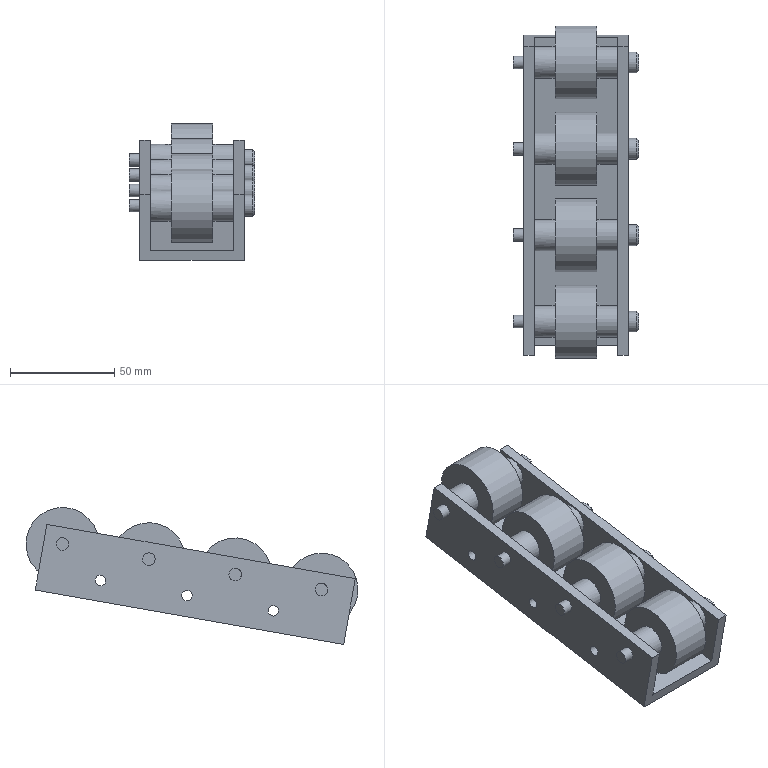Part | NX | features solid 2 | 1 solid | 56 faces | box 60 x 159.086 x 65.62 mm | volume 170595 mm3 | plane 26 | cylinder 26 | cone 4 | commonest cylinder face diameters 15 x8 5 x6 6 x4 10 x4 35 x4
STEP:
#1=CARTESIAN_POINT('',(-385.,-375.046,1.735));
#2=VERTEX_POINT('',#1);
#3=CARTESIAN_POINT('',(-385.,-374.612,-0.7271));
#4=DIRECTION('',(-1.,0.,0.));
#5=DIRECTION('',(0.,-0.1736,0.9848));
#6=AXIS2_PLACEMENT_3D('',#3,#4,#5);
#7=CIRCLE('',#6,2.5);
#8=EDGE_CURVE('',#2,#2,#7,.F.);
#9=ORIENTED_EDGE('',*,*,#8,.F.);
#10=EDGE_LOOP('',(#9));
#11=FACE_BOUND('',#10,.T.);
#12=CARTESIAN_POINT('',(-385.,-357.664,24.093));
#13=VERTEX_POINT('',#12);
#14=CARTESIAN_POINT('',(-385.,-356.362,16.707));
#15=DIRECTION('',(-1.,0.,0.));
#16=DIRECTION('',(0.,-0.1736,0.9848));
#17=AXIS2_PLACEMENT_3D('',#14,#15,#16);
#18=CIRCLE('',#17,7.5);
#19=EDGE_CURVE('',#13,#13,#18,.F.);
#20=ORIENTED_EDGE('',*,*,#19,.F.);
#21=EDGE_LOOP('',(#20));
#22=FACE_BOUND('',#21,.T.);
#23=CARTESIAN_POINT('',(-385.,-440.388,9.506));
#24=VERTEX_POINT('',#23);
#25=CARTESIAN_POINT('',(-385.,-439.086,2.12));
#26=DIRECTION('',(-1.,0.,0.));
#27=DIRECTION('',(0.,-0.1736,0.9848));
#28=AXIS2_PLACEMENT_3D('',#25,#26,#27);
#29=CIRCLE('',#28,7.5);
#30=EDGE_CURVE('',#24,#24,#29,.F.);
#31=ORIENTED_EDGE('',*,*,#30,.F.);
#32=EDGE_LOOP('',(#31));
#33=FACE_BOUND('',#32,.T.);
#34=CARTESIAN_POINT('',(-385.,-302.837,6.851));
#35=VERTEX_POINT('',#34);
#36=CARTESIAN_POINT('',(-385.,-307.526,33.441));
#37=VERTEX_POINT('',#36);
#38=CARTESIAN_POINT('',(-385.,-301.969,1.927));
#39=DIRECTION('',(0.,-0.1736,0.9848));
#40=VECTOR('',#39,1000.);
#41=LINE('',#38,#40);
#42=EDGE_CURVE('',#35,#37,#41,.T.);
#43=ORIENTED_EDGE('',*,*,#42,.T.);
#44=CARTESIAN_POINT('',(-385.,-455.247,7.394));
#45=VERTEX_POINT('',#44);
#46=CARTESIAN_POINT('',(-385.,-455.247,7.394));
#47=DIRECTION('',(0.,0.9848,0.1736));
#48=VECTOR('',#47,1000.);
#49=LINE('',#46,#48);
#50=EDGE_CURVE('',#45,#37,#49,.T.);
#51=ORIENTED_EDGE('',*,*,#50,.F.);
#52=CARTESIAN_POINT('',(-385.,-450.559,-19.196));
#53=VERTEX_POINT('',#52);
#54=CARTESIAN_POINT('',(-385.,-449.69,-24.12));
#55=DIRECTION('',(0.,-0.1736,0.9848));
#56=VECTOR('',#55,1000.);
#57=LINE('',#54,#56);
#58=EDGE_CURVE('',#53,#45,#57,.T.);
#59=ORIENTED_EDGE('',*,*,#58,.F.);
#60=CARTESIAN_POINT('',(-385.,-450.559,-19.196));
#61=DIRECTION('',(0.,0.9848,0.1736));
#62=VECTOR('',#61,1000.);
#63=LINE('',#60,#62);
#64=EDGE_CURVE('',#53,#35,#63,.T.);
#65=ORIENTED_EDGE('',*,*,#64,.T.);
#66=EDGE_LOOP('',(#43,#51,#59,#65));
#67=FACE_BOUND('',#66,.T.);
#68=CARTESIAN_POINT('',(-385.,-416.408,-5.558));
#69=VERTEX_POINT('',#68);
#70=CARTESIAN_POINT('',(-385.,-415.974,-8.02));
#71=DIRECTION('',(-1.,0.,0.));
#72=DIRECTION('',(0.,-0.1736,0.9848));
#73=AXIS2_PLACEMENT_3D('',#70,#71,#72);
#74=CIRCLE('',#73,2.5);
#75=EDGE_CURVE('',#69,#69,#74,.F.);
#76=ORIENTED_EDGE('',*,*,#75,.F.);
#77=EDGE_LOOP('',(#76));
#78=FACE_BOUND('',#77,.T.);
#79=CARTESIAN_POINT('',(-385.,-399.026,16.8));
#80=VERTEX_POINT('',#79);
#81=CARTESIAN_POINT('',(-385.,-397.724,9.414));
#82=DIRECTION('',(-1.,0.,0.));
#83=DIRECTION('',(0.,-0.1736,0.9848));
#84=AXIS2_PLACEMENT_3D('',#81,#82,#83);
#85=CIRCLE('',#84,7.5);
#86=EDGE_CURVE('',#80,#80,#85,.F.);
#87=ORIENTED_EDGE('',*,*,#86,.F.);
#88=EDGE_LOOP('',(#87));
#89=FACE_BOUND('',#88,.T.);
#90=CARTESIAN_POINT('',(-385.,-316.302,31.386));
#91=VERTEX_POINT('',#90);
#92=CARTESIAN_POINT('',(-385.,-315.,24.));
#93=DIRECTION('',(-1.,0.,0.));
#94=DIRECTION('',(0.,-0.1736,0.9848));
#95=AXIS2_PLACEMENT_3D('',#92,#93,#94);
#96=CIRCLE('',#95,7.5);
#97=EDGE_CURVE('',#91,#91,#96,.F.);
#98=ORIENTED_EDGE('',*,*,#97,.F.);
#99=EDGE_LOOP('',(#98));
#100=FACE_BOUND('',#99,.T.);
#101=CARTESIAN_POINT('',(-385.,-333.684,9.028));
#102=VERTEX_POINT('',#101);
#103=CARTESIAN_POINT('',(-385.,-333.25,6.566));
#104=DIRECTION('',(-1.,0.,0.));
#105=DIRECTION('',(0.,-0.1736,0.9848));
#106=AXIS2_PLACEMENT_3D('',#103,#104,#105);
#107=CIRCLE('',#106,2.5);
#108=EDGE_CURVE('',#102,#102,#107,.F.);
#109=ORIENTED_EDGE('',*,*,#108,.F.);
#110=EDGE_LOOP('',(#109));
#111=FACE_BOUND('',#110,.T.);
#112=CARTESIAN_POINT('',(-385.,-449.69,-24.12));
#113=DIRECTION('',(-1.,0.,0.));
#114=DIRECTION('',(0.,-0.1736,0.9848));
#115=AXIS2_PLACEMENT_3D('',#112,#113,#114);
#116=PLANE('',#115);
#117=ADVANCED_FACE('',(#11,#22,#33,#67,#78,#89,#100,#111),#116,.F.);
#118=CARTESIAN_POINT('',(-345.,-374.178,-3.189));
#119=VERTEX_POINT('',#118);
#120=CARTESIAN_POINT('',(-345.,-374.612,-0.7271));
#121=DIRECTION('',(1.,0.,0.));
#122=DIRECTION('',(0.,0.1736,-0.9848));
#123=AXIS2_PLACEMENT_3D('',#120,#121,#122);
#124=CIRCLE('',#123,2.5);
#125=EDGE_CURVE('',#119,#119,#124,.F.);
#126=ORIENTED_EDGE('',*,*,#125,.F.);
#127=EDGE_LOOP('',(#126));
#128=FACE_BOUND('',#127,.T.);
#129=CARTESIAN_POINT('',(-345.,-307.614,25.302));
#130=VERTEX_POINT('',#129);
#131=CARTESIAN_POINT('',(-345.,-315.,24.));
#132=DIRECTION('',(-1.,0.,0.));
#133=DIRECTION('',(0.,0.9848,0.1736));
#134=AXIS2_PLACEMENT_3D('',#131,#132,#133);
#135=CIRCLE('',#134,7.5);
#136=EDGE_CURVE('',#130,#130,#135,.T.);
#137=ORIENTED_EDGE('',*,*,#136,.F.);
#138=EDGE_LOOP('',(#137));
#139=FACE_BOUND('',#138,.T.);
#140=CARTESIAN_POINT('',(-345.,-348.976,18.009));
#141=VERTEX_POINT('',#140);
#142=CARTESIAN_POINT('',(-345.,-356.362,16.707));
#143=DIRECTION('',(-1.,0.,0.));
#144=DIRECTION('',(0.,0.9848,0.1736));
#145=AXIS2_PLACEMENT_3D('',#142,#143,#144);
#146=CIRCLE('',#145,7.5);
#147=EDGE_CURVE('',#141,#141,#146,.T.);
#148=ORIENTED_EDGE('',*,*,#147,.F.);
#149=EDGE_LOOP('',(#148));
#150=FACE_BOUND('',#149,.T.);
#151=CARTESIAN_POINT('',(-345.,-390.338,10.716));
#152=VERTEX_POINT('',#151);
#153=CARTESIAN_POINT('',(-345.,-397.724,9.414));
#154=DIRECTION('',(-1.,0.,0.));
#155=DIRECTION('',(0.,0.9848,0.1736));
#156=AXIS2_PLACEMENT_3D('',#153,#154,#155);
#157=CIRCLE('',#156,7.5);
#158=EDGE_CURVE('',#152,#152,#157,.T.);
#159=ORIENTED_EDGE('',*,*,#158,.F.);
#160=EDGE_LOOP('',(#159));
#161=FACE_BOUND('',#160,.T.);
#162=CARTESIAN_POINT('',(-345.,-415.54,-10.482));
#163=VERTEX_POINT('',#162);
#164=CARTESIAN_POINT('',(-345.,-415.974,-8.02));
#165=DIRECTION('',(1.,0.,0.));
#166=DIRECTION('',(0.,0.1736,-0.9848));
#167=AXIS2_PLACEMENT_3D('',#164,#165,#166);
#168=CIRCLE('',#167,2.5);
#169=EDGE_CURVE('',#163,#163,#168,.F.);
#170=ORIENTED_EDGE('',*,*,#169,.F.);
#171=EDGE_LOOP('',(#170));
#172=FACE_BOUND('',#171,.T.);
#173=CARTESIAN_POINT('',(-345.,-431.7,3.423));
#174=VERTEX_POINT('',#173);
#175=CARTESIAN_POINT('',(-345.,-439.086,2.12));
#176=DIRECTION('',(-1.,0.,0.));
#177=DIRECTION('',(0.,0.9848,0.1736));
#178=AXIS2_PLACEMENT_3D('',#175,#176,#177);
#179=CIRCLE('',#178,7.5);
#180=EDGE_CURVE('',#174,#174,#179,.T.);
#181=ORIENTED_EDGE('',*,*,#180,.F.);
#182=EDGE_LOOP('',(#181));
#183=FACE_BOUND('',#182,.T.);
#184=CARTESIAN_POINT('',(-345.,-307.526,33.441));
#185=VERTEX_POINT('',#184);
#186=CARTESIAN_POINT('',(-345.,-302.837,6.851));
#187=VERTEX_POINT('',#186);
#188=CARTESIAN_POINT('',(-345.,-307.526,33.441));
#189=DIRECTION('',(0.,0.1736,-0.9848));
#190=VECTOR('',#189,1000.);
#191=LINE('',#188,#190);
#192=EDGE_CURVE('',#185,#187,#191,.T.);
#193=ORIENTED_EDGE('',*,*,#192,.T.);
#194=CARTESIAN_POINT('',(-345.,-450.559,-19.196));
#195=VERTEX_POINT('',#194);
#196=CARTESIAN_POINT('',(-345.,-450.559,-19.196));
#197=DIRECTION('',(0.,0.9848,0.1736));
#198=VECTOR('',#197,1000.);
#199=LINE('',#196,#198);
#200=EDGE_CURVE('',#195,#187,#199,.T.);
#201=ORIENTED_EDGE('',*,*,#200,.F.);
#202=CARTESIAN_POINT('',(-345.,-455.247,7.394));
#203=VERTEX_POINT('',#202);
#204=CARTESIAN_POINT('',(-345.,-455.247,7.394));
#205=DIRECTION('',(0.,0.1736,-0.9848));
#206=VECTOR('',#205,1000.);
#207=LINE('',#204,#206);
#208=EDGE_CURVE('',#203,#195,#207,.T.);
#209=ORIENTED_EDGE('',*,*,#208,.F.);
#210=CARTESIAN_POINT('',(-345.,-455.247,7.394));
#211=DIRECTION('',(0.,0.9848,0.1736));
#212=VECTOR('',#211,1000.);
#213=LINE('',#210,#212);
#214=EDGE_CURVE('',#203,#185,#213,.T.);
#215=ORIENTED_EDGE('',*,*,#214,.T.);
#216=EDGE_LOOP('',(#193,#201,#209,#215));
#217=FACE_BOUND('',#216,.T.);
#218=CARTESIAN_POINT('',(-345.,-332.816,4.104));
#219=VERTEX_POINT('',#218);
#220=CARTESIAN_POINT('',(-345.,-333.25,6.566));
#221=DIRECTION('',(1.,0.,0.));
#222=DIRECTION('',(0.,0.1736,-0.9848));
#223=AXIS2_PLACEMENT_3D('',#220,#221,#222);
#224=CIRCLE('',#223,2.5);
#225=EDGE_CURVE('',#219,#219,#224,.F.);
#226=ORIENTED_EDGE('',*,*,#225,.F.);
#227=EDGE_LOOP('',(#226));
#228=FACE_BOUND('',#227,.T.);
#229=CARTESIAN_POINT('',(-345.,-455.247,7.394));
#230=DIRECTION('',(1.,0.,0.));
#231=DIRECTION('',(0.,0.1736,-0.9848));
#232=AXIS2_PLACEMENT_3D('',#229,#230,#231);
#233=PLANE('',#232);
#234=ADVANCED_FACE('',(#128,#139,#150,#161,#172,#183,#217,#228),#233,.F.);
#235=CARTESIAN_POINT('',(-390.,-375.046,1.735));
#236=VERTEX_POINT('',#235);
#237=CARTESIAN_POINT('',(-390.,-374.612,-0.7271));
#238=DIRECTION('',(-1.,0.,0.));
#239=DIRECTION('',(0.,-0.1736,0.9848));
#240=AXIS2_PLACEMENT_3D('',#237,#238,#239);
#241=CIRCLE('',#240,2.5);
#242=EDGE_CURVE('',#236,#236,#241,.F.);
#243=ORIENTED_EDGE('',*,*,#242,.T.);
#244=EDGE_LOOP('',(#243));
#245=FACE_BOUND('',#244,.T.);
#246=CARTESIAN_POINT('',(-390.,-356.883,19.661));
#247=VERTEX_POINT('',#246);
#248=CARTESIAN_POINT('',(-390.,-356.362,16.707));
#249=DIRECTION('',(-1.,0.,0.));
#250=DIRECTION('',(0.,-0.1736,0.9848));
#251=AXIS2_PLACEMENT_3D('',#248,#249,#250);
#252=CIRCLE('',#251,3.);
#253=EDGE_CURVE('',#247,#247,#252,.F.);
#254=ORIENTED_EDGE('',*,*,#253,.T.);
#255=EDGE_LOOP('',(#254));
#256=FACE_BOUND('',#255,.T.);
#257=CARTESIAN_POINT('',(-390.,-416.408,-5.558));
#258=VERTEX_POINT('',#257);
#259=CARTESIAN_POINT('',(-390.,-415.974,-8.02));
#260=DIRECTION('',(-1.,0.,0.));
#261=DIRECTION('',(0.,-0.1736,0.9848));
#262=AXIS2_PLACEMENT_3D('',#259,#260,#261);
#263=CIRCLE('',#262,2.5);
#264=EDGE_CURVE('',#258,#258,#263,.F.);
#265=ORIENTED_EDGE('',*,*,#264,.T.);
#266=EDGE_LOOP('',(#265));
#267=FACE_BOUND('',#266,.T.);
#268=CARTESIAN_POINT('',(-390.,-301.969,1.927));
#269=VERTEX_POINT('',#268);
#270=CARTESIAN_POINT('',(-390.,-307.526,33.441));
#271=VERTEX_POINT('',#270);
#272=CARTESIAN_POINT('',(-390.,-301.969,1.927));
#273=DIRECTION('',(0.,-0.1736,0.9848));
#274=VECTOR('',#273,1000.);
#275=LINE('',#272,#274);
#276=EDGE_CURVE('',#269,#271,#275,.T.);
#277=ORIENTED_EDGE('',*,*,#276,.F.);
#278=CARTESIAN_POINT('',(-390.,-449.69,-24.12));
#279=VERTEX_POINT('',#278);
#280=CARTESIAN_POINT('',(-390.,-449.69,-24.12));
#281=DIRECTION('',(0.,0.9848,0.1736));
#282=VECTOR('',#281,1000.);
#283=LINE('',#280,#282);
#284=EDGE_CURVE('',#279,#269,#283,.T.);
#285=ORIENTED_EDGE('',*,*,#284,.F.);
#286=CARTESIAN_POINT('',(-390.,-455.247,7.394));
#287=VERTEX_POINT('',#286);
#288=CARTESIAN_POINT('',(-390.,-449.69,-24.12));
#289=DIRECTION('',(0.,-0.1736,0.9848));
#290=VECTOR('',#289,1000.);
#291=LINE('',#288,#290);
#292=EDGE_CURVE('',#279,#287,#291,.T.);
#293=ORIENTED_EDGE('',*,*,#292,.T.);
#294=CARTESIAN_POINT('',(-390.,-455.247,7.394));
#295=DIRECTION('',(0.,0.9848,0.1736));
#296=VECTOR('',#295,1000.);
#297=LINE('',#294,#296);
#298=EDGE_CURVE('',#287,#271,#297,.T.);
#299=ORIENTED_EDGE('',*,*,#298,.T.);
#300=EDGE_LOOP('',(#277,#285,#293,#299));
#301=FACE_BOUND('',#300,.T.);
#302=CARTESIAN_POINT('',(-390.,-439.607,5.075));
#303=VERTEX_POINT('',#302);
#304=CARTESIAN_POINT('',(-390.,-439.086,2.12));
#305=DIRECTION('',(-1.,0.,0.));
#306=DIRECTION('',(0.,-0.1736,0.9848));
#307=AXIS2_PLACEMENT_3D('',#304,#305,#306);
#308=CIRCLE('',#307,3.);
#309=EDGE_CURVE('',#303,#303,#308,.F.);
#310=ORIENTED_EDGE('',*,*,#309,.T.);
#311=EDGE_LOOP('',(#310));
#312=FACE_BOUND('',#311,.T.);
#313=CARTESIAN_POINT('',(-390.,-398.245,12.368));
#314=VERTEX_POINT('',#313);
#315=CARTESIAN_POINT('',(-390.,-397.724,9.414));
#316=DIRECTION('',(-1.,0.,0.));
#317=DIRECTION('',(0.,-0.1736,0.9848));
#318=AXIS2_PLACEMENT_3D('',#315,#316,#317);
#319=CIRCLE('',#318,3.);
#320=EDGE_CURVE('',#314,#314,#319,.F.);
#321=ORIENTED_EDGE('',*,*,#320,.T.);
#322=EDGE_LOOP('',(#321));
#323=FACE_BOUND('',#322,.T.);
#324=CARTESIAN_POINT('',(-390.,-315.521,26.954));
#325=VERTEX_POINT('',#324);
#326=CARTESIAN_POINT('',(-390.,-315.,24.));
#327=DIRECTION('',(-1.,0.,0.));
#328=DIRECTION('',(0.,-0.1736,0.9848));
#329=AXIS2_PLACEMENT_3D('',#326,#327,#328);
#330=CIRCLE('',#329,3.);
#331=EDGE_CURVE('',#325,#325,#330,.F.);
#332=ORIENTED_EDGE('',*,*,#331,.T.);
#333=EDGE_LOOP('',(#332));
#334=FACE_BOUND('',#333,.T.);
#335=CARTESIAN_POINT('',(-390.,-333.684,9.028));
#336=VERTEX_POINT('',#335);
#337=CARTESIAN_POINT('',(-390.,-333.25,6.566));
#338=DIRECTION('',(-1.,0.,0.));
#339=DIRECTION('',(0.,-0.1736,0.9848));
#340=AXIS2_PLACEMENT_3D('',#337,#338,#339);
#341=CIRCLE('',#340,2.5);
#342=EDGE_CURVE('',#336,#336,#341,.F.);
#343=ORIENTED_EDGE('',*,*,#342,.T.);
#344=EDGE_LOOP('',(#343));
#345=FACE_BOUND('',#344,.T.);
#346=CARTESIAN_POINT('',(-390.,-449.69,-24.12));
#347=DIRECTION('',(-1.,0.,0.));
#348=DIRECTION('',(0.,-0.1736,0.9848));
#349=AXIS2_PLACEMENT_3D('',#346,#347,#348);
#350=PLANE('',#349);
#351=ADVANCED_FACE('',(#245,#256,#267,#301,#312,#323,#334,#345),#350,.T.);
#352=CARTESIAN_POINT('',(-340.,-374.178,-3.189));
#353=VERTEX_POINT('',#352);
#354=CARTESIAN_POINT('',(-340.,-374.612,-0.7271));
#355=DIRECTION('',(1.,0.,0.));
#356=DIRECTION('',(0.,0.1736,-0.9848));
#357=AXIS2_PLACEMENT_3D('',#354,#355,#356);
#358=CIRCLE('',#357,2.5);
#359=EDGE_CURVE('',#353,#353,#358,.F.);
#360=ORIENTED_EDGE('',*,*,#359,.T.);
#361=EDGE_LOOP('',(#360));
#362=FACE_BOUND('',#361,.T.);
#363=CARTESIAN_POINT('',(-340.,-314.132,19.076));
#364=VERTEX_POINT('',#363);
#365=CARTESIAN_POINT('',(-340.,-315.,24.));
#366=DIRECTION('',(1.,0.,0.));
#367=DIRECTION('',(0.,0.1736,-0.9848));
#368=AXIS2_PLACEMENT_3D('',#365,#366,#367);
#369=CIRCLE('',#368,5.);
#370=EDGE_CURVE('',#364,#364,#369,.T.);
#371=ORIENTED_EDGE('',*,*,#370,.F.);
#372=EDGE_LOOP('',(#371));
#373=FACE_BOUND('',#372,.T.);
#374=CARTESIAN_POINT('',(-340.,-355.494,11.783));
#375=VERTEX_POINT('',#374);
#376=CARTESIAN_POINT('',(-340.,-356.362,16.707));
#377=DIRECTION('',(1.,0.,0.));
#378=DIRECTION('',(0.,0.1736,-0.9848));
#379=AXIS2_PLACEMENT_3D('',#376,#377,#378);
#380=CIRCLE('',#379,5.);
#381=EDGE_CURVE('',#375,#375,#380,.T.);
#382=ORIENTED_EDGE('',*,*,#381,.F.);
#383=EDGE_LOOP('',(#382));
#384=FACE_BOUND('',#383,.T.);
#385=CARTESIAN_POINT('',(-340.,-396.856,4.49));
#386=VERTEX_POINT('',#385);
#387=CARTESIAN_POINT('',(-340.,-397.724,9.414));
#388=DIRECTION('',(1.,0.,0.));
#389=DIRECTION('',(0.,0.1736,-0.9848));
#390=AXIS2_PLACEMENT_3D('',#387,#388,#389);
#391=CIRCLE('',#390,5.);
#392=EDGE_CURVE('',#386,#386,#391,.T.);
#393=ORIENTED_EDGE('',*,*,#392,.F.);
#394=EDGE_LOOP('',(#393));
#395=FACE_BOUND('',#394,.T.);
#396=CARTESIAN_POINT('',(-340.,-415.54,-10.482));
#397=VERTEX_POINT('',#396);
#398=CARTESIAN_POINT('',(-340.,-415.974,-8.02));
#399=DIRECTION('',(1.,0.,0.));
#400=DIRECTION('',(0.,0.1736,-0.9848));
#401=AXIS2_PLACEMENT_3D('',#398,#399,#400);
#402=CIRCLE('',#401,2.5);
#403=EDGE_CURVE('',#397,#397,#402,.F.);
#404=ORIENTED_EDGE('',*,*,#403,.T.);
#405=EDGE_LOOP('',(#404));
#406=FACE_BOUND('',#405,.T.);
#407=CARTESIAN_POINT('',(-340.,-438.218,-2.804));
#408=VERTEX_POINT('',#407);
#409=CARTESIAN_POINT('',(-340.,-439.086,2.12));
#410=DIRECTION('',(1.,0.,0.));
#411=DIRECTION('',(0.,0.1736,-0.9848));
#412=AXIS2_PLACEMENT_3D('',#409,#410,#411);
#413=CIRCLE('',#412,5.);
#414=EDGE_CURVE('',#408,#408,#413,.T.);
#415=ORIENTED_EDGE('',*,*,#414,.F.);
#416=EDGE_LOOP('',(#415));
#417=FACE_BOUND('',#416,.T.);
#418=CARTESIAN_POINT('',(-340.,-307.526,33.441));
#419=VERTEX_POINT('',#418);
#420=CARTESIAN_POINT('',(-340.,-301.969,1.927));
#421=VERTEX_POINT('',#420);
#422=CARTESIAN_POINT('',(-340.,-307.526,33.441));
#423=DIRECTION('',(0.,0.1736,-0.9848));
#424=VECTOR('',#423,1000.);
#425=LINE('',#422,#424);
#426=EDGE_CURVE('',#419,#421,#425,.T.);
#427=ORIENTED_EDGE('',*,*,#426,.F.);
#428=CARTESIAN_POINT('',(-340.,-455.247,7.394));
#429=VERTEX_POINT('',#428);
#430=CARTESIAN_POINT('',(-340.,-455.247,7.394));
#431=DIRECTION('',(0.,0.9848,0.1736));
#432=VECTOR('',#431,1000.);
#433=LINE('',#430,#432);
#434=EDGE_CURVE('',#429,#419,#433,.T.);
#435=ORIENTED_EDGE('',*,*,#434,.F.);
#436=CARTESIAN_POINT('',(-340.,-449.69,-24.12));
#437=VERTEX_POINT('',#436);
#438=CARTESIAN_POINT('',(-340.,-455.247,7.394));
#439=DIRECTION('',(0.,0.1736,-0.9848));
#440=VECTOR('',#439,1000.);
#441=LINE('',#438,#440);
#442=EDGE_CURVE('',#429,#437,#441,.T.);
#443=ORIENTED_EDGE('',*,*,#442,.T.);
#444=CARTESIAN_POINT('',(-340.,-449.69,-24.12));
#445=DIRECTION('',(0.,0.9848,0.1736));
#446=VECTOR('',#445,1000.);
#447=LINE('',#444,#446);
#448=EDGE_CURVE('',#437,#421,#447,.T.);
#449=ORIENTED_EDGE('',*,*,#448,.T.);
#450=EDGE_LOOP('',(#427,#435,#443,#449));
#451=FACE_BOUND('',#450,.T.);
#452=CARTESIAN_POINT('',(-340.,-332.816,4.104));
#453=VERTEX_POINT('',#452);
#454=CARTESIAN_POINT('',(-340.,-333.25,6.566));
#455=DIRECTION('',(1.,0.,0.));
#456=DIRECTION('',(0.,0.1736,-0.9848));
#457=AXIS2_PLACEMENT_3D('',#454,#455,#456);
#458=CIRCLE('',#457,2.5);
#459=EDGE_CURVE('',#453,#453,#458,.F.);
#460=ORIENTED_EDGE('',*,*,#459,.T.);
#461=EDGE_LOOP('',(#460));
#462=FACE_BOUND('',#461,.T.);
#463=CARTESIAN_POINT('',(-340.,-455.247,7.394));
#464=DIRECTION('',(1.,0.,0.));
#465=DIRECTION('',(0.,0.1736,-0.9848));
#466=AXIS2_PLACEMENT_3D('',#463,#464,#465);
#467=PLANE('',#466);
#468=ADVANCED_FACE('',(#362,#373,#384,#395,#406,#417,#451,#462),#467,.T.);
#469=CARTESIAN_POINT('',(-375.,-297.766,27.039));
#470=VERTEX_POINT('',#469);
#471=CARTESIAN_POINT('',(-375.,-315.,24.));
#472=DIRECTION('',(-1.,0.,0.));
#473=DIRECTION('',(0.,0.9848,0.1736));
#474=AXIS2_PLACEMENT_3D('',#471,#472,#473);
#475=CIRCLE('',#474,17.5);
#476=EDGE_CURVE('',#470,#470,#475,.T.);
#477=ORIENTED_EDGE('',*,*,#476,.T.);
#478=EDGE_LOOP('',(#477));
#479=FACE_BOUND('',#478,.T.);
#480=CARTESIAN_POINT('',(-375.,-307.614,25.302));
#481=VERTEX_POINT('',#480);
#482=CARTESIAN_POINT('',(-375.,-315.,24.));
#483=DIRECTION('',(-1.,0.,0.));
#484=DIRECTION('',(0.,0.9848,0.1736));
#485=AXIS2_PLACEMENT_3D('',#482,#483,#484);
#486=CIRCLE('',#485,7.5);
#487=EDGE_CURVE('',#481,#481,#486,.T.);
#488=ORIENTED_EDGE('',*,*,#487,.F.);
#489=EDGE_LOOP('',(#488));
#490=FACE_BOUND('',#489,.T.);
#491=CARTESIAN_POINT('',(-375.,-315.,24.));
#492=DIRECTION('',(-1.,0.,0.));
#493=DIRECTION('',(0.,-0.1736,0.9848));
#494=AXIS2_PLACEMENT_3D('',#491,#492,#493);
#495=PLANE('',#494);
#496=ADVANCED_FACE('',(#479,#490),#495,.T.);
#497=CARTESIAN_POINT('',(-375.,-339.128,19.746));
#498=VERTEX_POINT('',#497);
#499=CARTESIAN_POINT('',(-375.,-356.362,16.707));
#500=DIRECTION('',(-1.,0.,0.));
#501=DIRECTION('',(0.,0.9848,0.1736));
#502=AXIS2_PLACEMENT_3D('',#499,#500,#501);
#503=CIRCLE('',#502,17.5);
#504=EDGE_CURVE('',#498,#498,#503,.T.);
#505=ORIENTED_EDGE('',*,*,#504,.T.);
#506=EDGE_LOOP('',(#505));
#507=FACE_BOUND('',#506,.T.);
#508=CARTESIAN_POINT('',(-375.,-348.976,18.009));
#509=VERTEX_POINT('',#508);
#510=CARTESIAN_POINT('',(-375.,-356.362,16.707));
#511=DIRECTION('',(-1.,0.,0.));
#512=DIRECTION('',(0.,0.9848,0.1736));
#513=AXIS2_PLACEMENT_3D('',#510,#511,#512);
#514=CIRCLE('',#513,7.5);
#515=EDGE_CURVE('',#509,#509,#514,.T.);
#516=ORIENTED_EDGE('',*,*,#515,.F.);
#517=EDGE_LOOP('',(#516));
#518=FACE_BOUND('',#517,.T.);
#519=CARTESIAN_POINT('',(-375.,-356.362,16.707));
#520=DIRECTION('',(-1.,0.,0.));
#521=DIRECTION('',(0.,-0.1736,0.9848));
#522=AXIS2_PLACEMENT_3D('',#519,#520,#521);
#523=PLANE('',#522);
#524=ADVANCED_FACE('',(#507,#518),#523,.T.);
#525=CARTESIAN_POINT('',(-375.,-380.49,12.452));
#526=VERTEX_POINT('',#525);
#527=CARTESIAN_POINT('',(-375.,-397.724,9.414));
#528=DIRECTION('',(-1.,0.,0.));
#529=DIRECTION('',(0.,0.9848,0.1736));
#530=AXIS2_PLACEMENT_3D('',#527,#528,#529);
#531=CIRCLE('',#530,17.5);
#532=EDGE_CURVE('',#526,#526,#531,.T.);
#533=ORIENTED_EDGE('',*,*,#532,.T.);
#534=EDGE_LOOP('',(#533));
#535=FACE_BOUND('',#534,.T.);
#536=CARTESIAN_POINT('',(-375.,-390.338,10.716));
#537=VERTEX_POINT('',#536);
#538=CARTESIAN_POINT('',(-375.,-397.724,9.414));
#539=DIRECTION('',(-1.,0.,0.));
#540=DIRECTION('',(0.,0.9848,0.1736));
#541=AXIS2_PLACEMENT_3D('',#538,#539,#540);
#542=CIRCLE('',#541,7.5);
#543=EDGE_CURVE('',#537,#537,#542,.T.);
#544=ORIENTED_EDGE('',*,*,#543,.F.);
#545=EDGE_LOOP('',(#544));
#546=FACE_BOUND('',#545,.T.);
#547=CARTESIAN_POINT('',(-375.,-397.724,9.414));
#548=DIRECTION('',(-1.,0.,0.));
#549=DIRECTION('',(0.,-0.1736,0.9848));
#550=AXIS2_PLACEMENT_3D('',#547,#548,#549);
#551=PLANE('',#550);
#552=ADVANCED_FACE('',(#535,#546),#551,.T.);
#553=CARTESIAN_POINT('',(-375.,-421.852,5.159));
#554=VERTEX_POINT('',#553);
#555=CARTESIAN_POINT('',(-375.,-439.086,2.12));
#556=DIRECTION('',(-1.,0.,0.));
#557=DIRECTION('',(0.,0.9848,0.1736));
#558=AXIS2_PLACEMENT_3D('',#555,#556,#557);
#559=CIRCLE('',#558,17.5);
#560=EDGE_CURVE('',#554,#554,#559,.T.);
#561=ORIENTED_EDGE('',*,*,#560,.T.);
#562=EDGE_LOOP('',(#561));
#563=FACE_BOUND('',#562,.T.);
#564=CARTESIAN_POINT('',(-375.,-431.7,3.423));
#565=VERTEX_POINT('',#564);
#566=CARTESIAN_POINT('',(-375.,-439.086,2.12));
#567=DIRECTION('',(-1.,0.,0.));
#568=DIRECTION('',(0.,0.9848,0.1736));
#569=AXIS2_PLACEMENT_3D('',#566,#567,#568);
#570=CIRCLE('',#569,7.5);
#571=EDGE_CURVE('',#565,#565,#570,.T.);
#572=ORIENTED_EDGE('',*,*,#571,.F.);
#573=EDGE_LOOP('',(#572));
#574=FACE_BOUND('',#573,.T.);
#575=CARTESIAN_POINT('',(-375.,-439.086,2.12));
#576=DIRECTION('',(-1.,0.,0.));
#577=DIRECTION('',(0.,-0.1736,0.9848));
#578=AXIS2_PLACEMENT_3D('',#575,#576,#577);
#579=PLANE('',#578);
#580=ADVANCED_FACE('',(#563,#574),#579,.T.);
#581=ORIENTED_EDGE('',*,*,#208,.T.);
#582=CARTESIAN_POINT('',(-340.,-450.559,-19.196));
#583=DIRECTION('',(-1.,0.,0.));
#584=VECTOR('',#583,1000.);
#585=LINE('',#582,#584);
#586=EDGE_CURVE('',#195,#53,#585,.T.);
#587=ORIENTED_EDGE('',*,*,#586,.T.);
#588=ORIENTED_EDGE('',*,*,#58,.T.);
#589=CARTESIAN_POINT('',(-390.,-455.247,7.394));
#590=DIRECTION('',(1.,0.,0.));
#591=VECTOR('',#590,1000.);
#592=LINE('',#589,#591);
#593=EDGE_CURVE('',#287,#45,#592,.T.);
#594=ORIENTED_EDGE('',*,*,#593,.F.);
#595=ORIENTED_EDGE('',*,*,#292,.F.);
#596=CARTESIAN_POINT('',(-340.,-449.69,-24.12));
#597=DIRECTION('',(-1.,0.,0.));
#598=VECTOR('',#597,1000.);
#599=LINE('',#596,#598);
#600=EDGE_CURVE('',#437,#279,#599,.T.);
#601=ORIENTED_EDGE('',*,*,#600,.F.);
#602=ORIENTED_EDGE('',*,*,#442,.F.);
#603=CARTESIAN_POINT('',(-340.,-455.247,7.394));
#604=DIRECTION('',(-1.,0.,0.));
#605=VECTOR('',#604,1000.);
#606=LINE('',#603,#605);
#607=EDGE_CURVE('',#429,#203,#606,.T.);
#608=ORIENTED_EDGE('',*,*,#607,.T.);
#609=EDGE_LOOP('',(#581,#587,#588,#594,#595,#601,#602,#608));
#610=FACE_BOUND('',#609,.T.);
#611=CARTESIAN_POINT('',(-340.,-455.247,7.394));
#612=DIRECTION('',(0.,-0.9848,-0.1736));
#613=DIRECTION('',(0.,0.1736,-0.9848));
#614=AXIS2_PLACEMENT_3D('',#611,#612,#613);
#615=PLANE('',#614);
#616=ADVANCED_FACE('',(#610),#615,.T.);
#617=ORIENTED_EDGE('',*,*,#607,.F.);
#618=ORIENTED_EDGE('',*,*,#434,.T.);
#619=CARTESIAN_POINT('',(-340.,-307.526,33.441));
#620=DIRECTION('',(-1.,0.,0.));
#621=VECTOR('',#620,1000.);
#622=LINE('',#619,#621);
#623=EDGE_CURVE('',#419,#185,#622,.T.);
#624=ORIENTED_EDGE('',*,*,#623,.T.);
#625=ORIENTED_EDGE('',*,*,#214,.F.);
#626=EDGE_LOOP('',(#617,#618,#624,#625));
#627=FACE_BOUND('',#626,.T.);
#628=CARTESIAN_POINT('',(-340.,-455.247,7.394));
#629=DIRECTION('',(0.,0.1736,-0.9848));
#630=DIRECTION('',(0.,0.9848,0.1736));
#631=AXIS2_PLACEMENT_3D('',#628,#629,#630);
#632=PLANE('',#631);
#633=ADVANCED_FACE('',(#627),#632,.F.);
#634=ORIENTED_EDGE('',*,*,#42,.F.);
#635=CARTESIAN_POINT('',(-340.,-302.837,6.851));
#636=DIRECTION('',(-1.,0.,0.));
#637=VECTOR('',#636,1000.);
#638=LINE('',#635,#637);
#639=EDGE_CURVE('',#187,#35,#638,.T.);
#640=ORIENTED_EDGE('',*,*,#639,.F.);
#641=ORIENTED_EDGE('',*,*,#192,.F.);
#642=ORIENTED_EDGE('',*,*,#623,.F.);
#643=ORIENTED_EDGE('',*,*,#426,.T.);
#644=CARTESIAN_POINT('',(-340.,-301.969,1.927));
#645=DIRECTION('',(-1.,0.,0.));
#646=VECTOR('',#645,1000.);
#647=LINE('',#644,#646);
#648=EDGE_CURVE('',#421,#269,#647,.T.);
#649=ORIENTED_EDGE('',*,*,#648,.T.);
#650=ORIENTED_EDGE('',*,*,#276,.T.);
#651=CARTESIAN_POINT('',(-390.,-307.526,33.441));
#652=DIRECTION('',(1.,0.,0.));
#653=VECTOR('',#652,1000.);
#654=LINE('',#651,#653);
#655=EDGE_CURVE('',#271,#37,#654,.T.);
#656=ORIENTED_EDGE('',*,*,#655,.T.);
#657=EDGE_LOOP('',(#634,#640,#641,#642,#643,#649,#650,#656));
#658=FACE_BOUND('',#657,.T.);
#659=CARTESIAN_POINT('',(-390.,-301.969,1.927));
#660=DIRECTION('',(0.,-0.9848,-0.1736));
#661=DIRECTION('',(0.,-0.1736,0.9848));
#662=AXIS2_PLACEMENT_3D('',#659,#660,#661);
#663=PLANE('',#662);
#664=ADVANCED_FACE('',(#658),#663,.F.);
#665=ORIENTED_EDGE('',*,*,#639,.T.);
#666=ORIENTED_EDGE('',*,*,#64,.F.);
#667=ORIENTED_EDGE('',*,*,#586,.F.);
#668=ORIENTED_EDGE('',*,*,#200,.T.);
#669=EDGE_LOOP('',(#665,#666,#667,#668));
#670=FACE_BOUND('',#669,.T.);
#671=CARTESIAN_POINT('',(-340.,-450.559,-19.196));
#672=DIRECTION('',(0.,0.1736,-0.9848));
#673=DIRECTION('',(0.,-0.9848,-0.1736));
#674=AXIS2_PLACEMENT_3D('',#671,#672,#673);
#675=PLANE('',#674);
#676=ADVANCED_FACE('',(#670),#675,.F.);
#677=ORIENTED_EDGE('',*,*,#298,.F.);
#678=ORIENTED_EDGE('',*,*,#593,.T.);
#679=ORIENTED_EDGE('',*,*,#50,.T.);
#680=ORIENTED_EDGE('',*,*,#655,.F.);
#681=EDGE_LOOP('',(#677,#678,#679,#680));
#682=FACE_BOUND('',#681,.T.);
#683=CARTESIAN_POINT('',(-390.,-455.247,7.394));
#684=DIRECTION('',(0.,-0.1736,0.9848));
#685=DIRECTION('',(0.,0.9848,0.1736));
#686=AXIS2_PLACEMENT_3D('',#683,#684,#685);
#687=PLANE('',#686);
#688=ADVANCED_FACE('',(#682),#687,.T.);
#689=ORIENTED_EDGE('',*,*,#648,.F.);
#690=ORIENTED_EDGE('',*,*,#448,.F.);
#691=ORIENTED_EDGE('',*,*,#600,.T.);
#692=ORIENTED_EDGE('',*,*,#284,.T.);
#693=EDGE_LOOP('',(#689,#690,#691,#692));
#694=FACE_BOUND('',#693,.T.);
#695=CARTESIAN_POINT('',(-340.,-449.69,-24.12));
#696=DIRECTION('',(0.,0.1736,-0.9848));
#697=DIRECTION('',(0.,-0.9848,-0.1736));
#698=AXIS2_PLACEMENT_3D('',#695,#696,#697);
#699=PLANE('',#698);
#700=ADVANCED_FACE('',(#694),#699,.T.);
#701=CARTESIAN_POINT('',(-395.,-436.131,2.641));
#702=VERTEX_POINT('',#701);
#703=CARTESIAN_POINT('',(-395.,-439.086,2.12));
#704=DIRECTION('',(-1.,0.,0.));
#705=DIRECTION('',(0.,0.9848,0.1736));
#706=AXIS2_PLACEMENT_3D('',#703,#704,#705);
#707=CIRCLE('',#706,3.);
#708=EDGE_CURVE('',#702,#702,#707,.T.);
#709=ORIENTED_EDGE('',*,*,#708,.T.);
#710=EDGE_LOOP('',(#709));
#711=FACE_BOUND('',#710,.T.);
#712=CARTESIAN_POINT('',(-395.,-439.086,2.12));
#713=DIRECTION('',(-1.,0.,0.));
#714=DIRECTION('',(0.,-0.1736,0.9848));
#715=AXIS2_PLACEMENT_3D('',#712,#713,#714);
#716=PLANE('',#715);
#717=ADVANCED_FACE('',(#711),#716,.T.);
#718=ORIENTED_EDGE('',*,*,#309,.F.);
#719=EDGE_LOOP('',(#718));
#720=FACE_BOUND('',#719,.T.);
#721=ORIENTED_EDGE('',*,*,#708,.F.);
#722=EDGE_LOOP('',(#721));
#723=FACE_BOUND('',#722,.T.);
#724=CARTESIAN_POINT('',(-395.,-439.086,2.12));
#725=DIRECTION('',(1.,0.,0.));
#726=DIRECTION('',(0.,0.1736,-0.9848));
#727=AXIS2_PLACEMENT_3D('',#724,#725,#726);
#728=CYLINDRICAL_SURFACE('',#727,3.);
#729=ADVANCED_FACE('',(#720,#723),#728,.T.);
#730=CARTESIAN_POINT('',(-355.,-431.7,3.423));
#731=VERTEX_POINT('',#730);
#732=CARTESIAN_POINT('',(-355.,-439.086,2.12));
#733=DIRECTION('',(-1.,0.,0.));
#734=DIRECTION('',(0.,0.9848,0.1736));
#735=AXIS2_PLACEMENT_3D('',#732,#733,#734);
#736=CIRCLE('',#735,7.5);
#737=EDGE_CURVE('',#731,#731,#736,.T.);
#738=ORIENTED_EDGE('',*,*,#737,.T.);
#739=EDGE_LOOP('',(#738));
#740=FACE_BOUND('',#739,.T.);
#741=CARTESIAN_POINT('',(-355.,-421.852,5.159));
#742=VERTEX_POINT('',#741);
#743=CARTESIAN_POINT('',(-355.,-439.086,2.12));
#744=DIRECTION('',(-1.,0.,0.));
#745=DIRECTION('',(0.,0.9848,0.1736));
#746=AXIS2_PLACEMENT_3D('',#743,#744,#745);
#747=CIRCLE('',#746,17.5);
#748=EDGE_CURVE('',#742,#742,#747,.T.);
#749=ORIENTED_EDGE('',*,*,#748,.F.);
#750=EDGE_LOOP('',(#749));
#751=FACE_BOUND('',#750,.T.);
#752=CARTESIAN_POINT('',(-355.,-439.086,2.12));
#753=DIRECTION('',(-1.,0.,0.));
#754=DIRECTION('',(0.,-0.1736,0.9848));
#755=AXIS2_PLACEMENT_3D('',#752,#753,#754);
#756=PLANE('',#755);
#757=ADVANCED_FACE('',(#740,#751),#756,.F.);
#758=ORIENTED_EDGE('',*,*,#560,.F.);
#759=EDGE_LOOP('',(#758));
#760=FACE_BOUND('',#759,.T.);
#761=ORIENTED_EDGE('',*,*,#748,.T.);
#762=EDGE_LOOP('',(#761));
#763=FACE_BOUND('',#762,.T.);
#764=CARTESIAN_POINT('',(-375.,-439.086,2.12));
#765=DIRECTION('',(1.,0.,0.));
#766=DIRECTION('',(0.,0.1736,-0.9848));
#767=AXIS2_PLACEMENT_3D('',#764,#765,#766);
#768=CYLINDRICAL_SURFACE('',#767,17.5);
#769=ADVANCED_FACE('',(#760,#763),#768,.T.);
#770=ORIENTED_EDGE('',*,*,#30,.T.);
#771=EDGE_LOOP('',(#770));
#772=FACE_BOUND('',#771,.T.);
#773=ORIENTED_EDGE('',*,*,#571,.T.);
#774=EDGE_LOOP('',(#773));
#775=FACE_BOUND('',#774,.T.);
#776=CARTESIAN_POINT('',(-385.,-439.086,2.12));
#777=DIRECTION('',(1.,0.,0.));
#778=DIRECTION('',(0.,0.1736,-0.9848));
#779=AXIS2_PLACEMENT_3D('',#776,#777,#778);
#780=CYLINDRICAL_SURFACE('',#779,7.5);
#781=ADVANCED_FACE('',(#772,#775),#780,.T.);
#782=ORIENTED_EDGE('',*,*,#180,.T.);
#783=EDGE_LOOP('',(#782));
#784=FACE_BOUND('',#783,.T.);
#785=ORIENTED_EDGE('',*,*,#737,.F.);
#786=EDGE_LOOP('',(#785));
#787=FACE_BOUND('',#786,.T.);
#788=CARTESIAN_POINT('',(-345.,-439.086,2.12));
#789=DIRECTION('',(-1.,0.,0.));
#790=DIRECTION('',(0.,-0.1736,0.9848));
#791=AXIS2_PLACEMENT_3D('',#788,#789,#790);
#792=CYLINDRICAL_SURFACE('',#791,7.5);
#793=ADVANCED_FACE('',(#784,#787),#792,.T.);
#794=CARTESIAN_POINT('',(-336.,-439.954,7.044));
#795=VERTEX_POINT('',#794);
#796=CARTESIAN_POINT('',(-336.,-439.086,2.12));
#797=DIRECTION('',(-1.,0.,0.));
#798=DIRECTION('',(0.,-0.1736,0.9848));
#799=AXIS2_PLACEMENT_3D('',#796,#797,#798);
#800=CIRCLE('',#799,5.);
#801=EDGE_CURVE('',#795,#795,#800,.T.);
#802=ORIENTED_EDGE('',*,*,#801,.T.);
#803=EDGE_LOOP('',(#802));
#804=FACE_BOUND('',#803,.T.);
#805=ORIENTED_EDGE('',*,*,#414,.T.);
#806=EDGE_LOOP('',(#805));
#807=FACE_BOUND('',#806,.T.);
#808=CARTESIAN_POINT('',(-335.,-439.086,2.12));
#809=DIRECTION('',(-1.,0.,0.));
#810=DIRECTION('',(0.,-0.1736,0.9848));
#811=AXIS2_PLACEMENT_3D('',#808,#809,#810);
#812=CYLINDRICAL_SURFACE('',#811,5.);
#813=ADVANCED_FACE('',(#804,#807),#812,.T.);
#814=CARTESIAN_POINT('',(-335.,-439.78,6.06));
#815=VERTEX_POINT('',#814);
#816=CARTESIAN_POINT('',(-335.,-439.086,2.12));
#817=DIRECTION('',(-1.,0.,0.));
#818=DIRECTION('',(0.,-0.1736,0.9848));
#819=AXIS2_PLACEMENT_3D('',#816,#817,#818);
#820=CIRCLE('',#819,4.);
#821=EDGE_CURVE('',#815,#815,#820,.F.);
#822=ORIENTED_EDGE('',*,*,#821,.T.);
#823=EDGE_LOOP('',(#822));
#824=FACE_BOUND('',#823,.T.);
#825=CARTESIAN_POINT('',(-335.,-439.086,2.12));
#826=DIRECTION('',(-1.,0.,0.));
#827=DIRECTION('',(0.,-0.1736,0.9848));
#828=AXIS2_PLACEMENT_3D('',#825,#826,#827);
#829=PLANE('',#828);
#830=ADVANCED_FACE('',(#824),#829,.F.);
#831=ORIENTED_EDGE('',*,*,#403,.F.);
#832=EDGE_LOOP('',(#831));
#833=FACE_BOUND('',#832,.T.);
#834=ORIENTED_EDGE('',*,*,#169,.T.);
#835=EDGE_LOOP('',(#834));
#836=FACE_BOUND('',#835,.T.);
#837=CARTESIAN_POINT('',(-395.,-415.974,-8.02));
#838=DIRECTION('',(1.,0.,0.));
#839=DIRECTION('',(0.,0.1736,-0.9848));
#840=AXIS2_PLACEMENT_3D('',#837,#838,#839);
#841=CYLINDRICAL_SURFACE('',#840,2.5);
#842=ADVANCED_FACE('',(#833,#836),#841,.F.);
#843=ORIENTED_EDGE('',*,*,#264,.F.);
#844=EDGE_LOOP('',(#843));
#845=FACE_BOUND('',#844,.T.);
#846=ORIENTED_EDGE('',*,*,#75,.T.);
#847=EDGE_LOOP('',(#846));
#848=FACE_BOUND('',#847,.T.);
#849=CARTESIAN_POINT('',(-395.,-415.974,-8.02));
#850=DIRECTION('',(1.,0.,0.));
#851=DIRECTION('',(0.,0.1736,-0.9848));
#852=AXIS2_PLACEMENT_3D('',#849,#850,#851);
#853=CYLINDRICAL_SURFACE('',#852,2.5);
#854=ADVANCED_FACE('',(#845,#848),#853,.F.);
#855=CARTESIAN_POINT('',(-395.,-394.769,9.934));
#856=VERTEX_POINT('',#855);
#857=CARTESIAN_POINT('',(-395.,-397.724,9.414));
#858=DIRECTION('',(-1.,0.,0.));
#859=DIRECTION('',(0.,0.9848,0.1736));
#860=AXIS2_PLACEMENT_3D('',#857,#858,#859);
#861=CIRCLE('',#860,3.);
#862=EDGE_CURVE('',#856,#856,#861,.T.);
#863=ORIENTED_EDGE('',*,*,#862,.T.);
#864=EDGE_LOOP('',(#863));
#865=FACE_BOUND('',#864,.T.);
#866=CARTESIAN_POINT('',(-395.,-397.724,9.414));
#867=DIRECTION('',(-1.,0.,0.));
#868=DIRECTION('',(0.,-0.1736,0.9848));
#869=AXIS2_PLACEMENT_3D('',#866,#867,#868);
#870=PLANE('',#869);
#871=ADVANCED_FACE('',(#865),#870,.T.);
#872=ORIENTED_EDGE('',*,*,#320,.F.);
#873=EDGE_LOOP('',(#872));
#874=FACE_BOUND('',#873,.T.);
#875=ORIENTED_EDGE('',*,*,#862,.F.);
#876=EDGE_LOOP('',(#875));
#877=FACE_BOUND('',#876,.T.);
#878=CARTESIAN_POINT('',(-395.,-397.724,9.414));
#879=DIRECTION('',(1.,0.,0.));
#880=DIRECTION('',(0.,0.1736,-0.9848));
#881=AXIS2_PLACEMENT_3D('',#878,#879,#880);
#882=CYLINDRICAL_SURFACE('',#881,3.);
#883=ADVANCED_FACE('',(#874,#877),#882,.T.);
#884=CARTESIAN_POINT('',(-395.,-353.408,17.228));
#885=VERTEX_POINT('',#884);
#886=CARTESIAN_POINT('',(-395.,-356.362,16.707));
#887=DIRECTION('',(-1.,0.,0.));
#888=DIRECTION('',(0.,0.9848,0.1736));
#889=AXIS2_PLACEMENT_3D('',#886,#887,#888);
#890=CIRCLE('',#889,3.);
#891=EDGE_CURVE('',#885,#885,#890,.T.);
#892=ORIENTED_EDGE('',*,*,#891,.T.);
#893=EDGE_LOOP('',(#892));
#894=FACE_BOUND('',#893,.T.);
#895=CARTESIAN_POINT('',(-395.,-356.362,16.707));
#896=DIRECTION('',(-1.,0.,0.));
#897=DIRECTION('',(0.,-0.1736,0.9848));
#898=AXIS2_PLACEMENT_3D('',#895,#896,#897);
#899=PLANE('',#898);
#900=ADVANCED_FACE('',(#894),#899,.T.);
#901=ORIENTED_EDGE('',*,*,#253,.F.);
#902=EDGE_LOOP('',(#901));
#903=FACE_BOUND('',#902,.T.);
#904=ORIENTED_EDGE('',*,*,#891,.F.);
#905=EDGE_LOOP('',(#904));
#906=FACE_BOUND('',#905,.T.);
#907=CARTESIAN_POINT('',(-395.,-356.362,16.707));
#908=DIRECTION('',(1.,0.,0.));
#909=DIRECTION('',(0.,0.1736,-0.9848));
#910=AXIS2_PLACEMENT_3D('',#907,#908,#909);
#911=CYLINDRICAL_SURFACE('',#910,3.);
#912=ADVANCED_FACE('',(#903,#906),#911,.T.);
#913=CARTESIAN_POINT('',(-395.,-312.046,24.521));
#914=VERTEX_POINT('',#913);
#915=CARTESIAN_POINT('',(-395.,-315.,24.));
#916=DIRECTION('',(-1.,0.,0.));
#917=DIRECTION('',(0.,0.9848,0.1736));
#918=AXIS2_PLACEMENT_3D('',#915,#916,#917);
#919=CIRCLE('',#918,3.);
#920=EDGE_CURVE('',#914,#914,#919,.T.);
#921=ORIENTED_EDGE('',*,*,#920,.T.);
#922=EDGE_LOOP('',(#921));
#923=FACE_BOUND('',#922,.T.);
#924=CARTESIAN_POINT('',(-395.,-315.,24.));
#925=DIRECTION('',(-1.,0.,0.));
#926=DIRECTION('',(0.,-0.1736,0.9848));
#927=AXIS2_PLACEMENT_3D('',#924,#925,#926);
#928=PLANE('',#927);
#929=ADVANCED_FACE('',(#923),#928,.T.);
#930=ORIENTED_EDGE('',*,*,#331,.F.);
#931=EDGE_LOOP('',(#930));
#932=FACE_BOUND('',#931,.T.);
#933=ORIENTED_EDGE('',*,*,#920,.F.);
#934=EDGE_LOOP('',(#933));
#935=FACE_BOUND('',#934,.T.);
#936=CARTESIAN_POINT('',(-395.,-315.,24.));
#937=DIRECTION('',(1.,0.,0.));
#938=DIRECTION('',(0.,0.1736,-0.9848));
#939=AXIS2_PLACEMENT_3D('',#936,#937,#938);
#940=CYLINDRICAL_SURFACE('',#939,3.);
#941=ADVANCED_FACE('',(#932,#935),#940,.T.);
#942=CARTESIAN_POINT('',(-355.,-390.338,10.716));
#943=VERTEX_POINT('',#942);
#944=CARTESIAN_POINT('',(-355.,-397.724,9.414));
#945=DIRECTION('',(-1.,0.,0.));
#946=DIRECTION('',(0.,0.9848,0.1736));
#947=AXIS2_PLACEMENT_3D('',#944,#945,#946);
#948=CIRCLE('',#947,7.5);
#949=EDGE_CURVE('',#943,#943,#948,.T.);
#950=ORIENTED_EDGE('',*,*,#949,.T.);
#951=EDGE_LOOP('',(#950));
#952=FACE_BOUND('',#951,.T.);
#953=CARTESIAN_POINT('',(-355.,-380.49,12.452));
#954=VERTEX_POINT('',#953);
#955=CARTESIAN_POINT('',(-355.,-397.724,9.414));
#956=DIRECTION('',(-1.,0.,0.));
#957=DIRECTION('',(0.,0.9848,0.1736));
#958=AXIS2_PLACEMENT_3D('',#955,#956,#957);
#959=CIRCLE('',#958,17.5);
#960=EDGE_CURVE('',#954,#954,#959,.T.);
#961=ORIENTED_EDGE('',*,*,#960,.F.);
#962=EDGE_LOOP('',(#961));
#963=FACE_BOUND('',#962,.T.);
#964=CARTESIAN_POINT('',(-355.,-397.724,9.414));
#965=DIRECTION('',(-1.,0.,0.));
#966=DIRECTION('',(0.,-0.1736,0.9848));
#967=AXIS2_PLACEMENT_3D('',#964,#965,#966);
#968=PLANE('',#967);
#969=ADVANCED_FACE('',(#952,#963),#968,.F.);
#970=ORIENTED_EDGE('',*,*,#532,.F.);
#971=EDGE_LOOP('',(#970));
#972=FACE_BOUND('',#971,.T.);
#973=ORIENTED_EDGE('',*,*,#960,.T.);
#974=EDGE_LOOP('',(#973));
#975=FACE_BOUND('',#974,.T.);
#976=CARTESIAN_POINT('',(-375.,-397.724,9.414));
#977=DIRECTION('',(1.,0.,0.));
#978=DIRECTION('',(0.,0.1736,-0.9848));
#979=AXIS2_PLACEMENT_3D('',#976,#977,#978);
#980=CYLINDRICAL_SURFACE('',#979,17.5);
#981=ADVANCED_FACE('',(#972,#975),#980,.T.);
#982=CARTESIAN_POINT('',(-355.,-348.976,18.009));
#983=VERTEX_POINT('',#982);
#984=CARTESIAN_POINT('',(-355.,-356.362,16.707));
#985=DIRECTION('',(-1.,0.,0.));
#986=DIRECTION('',(0.,0.9848,0.1736));
#987=AXIS2_PLACEMENT_3D('',#984,#985,#986);
#988=CIRCLE('',#987,7.5);
#989=EDGE_CURVE('',#983,#983,#988,.T.);
#990=ORIENTED_EDGE('',*,*,#989,.T.);
#991=EDGE_LOOP('',(#990));
#992=FACE_BOUND('',#991,.T.);
#993=CARTESIAN_POINT('',(-355.,-339.128,19.746));
#994=VERTEX_POINT('',#993);
#995=CARTESIAN_POINT('',(-355.,-356.362,16.707));
#996=DIRECTION('',(-1.,0.,0.));
#997=DIRECTION('',(0.,0.9848,0.1736));
#998=AXIS2_PLACEMENT_3D('',#995,#996,#997);
#999=CIRCLE('',#998,17.5);
#1000=EDGE_CURVE('',#994,#994,#999,.T.);
#1001=ORIENTED_EDGE('',*,*,#1000,.F.);
#1002=EDGE_LOOP('',(#1001));
#1003=FACE_BOUND('',#1002,.T.);
#1004=CARTESIAN_POINT('',(-355.,-356.362,16.707));
#1005=DIRECTION('',(-1.,0.,0.));
#1006=DIRECTION('',(0.,-0.1736,0.9848));
#1007=AXIS2_PLACEMENT_3D('',#1004,#1005,#1006);
#1008=PLANE('',#1007);
#1009=ADVANCED_FACE('',(#992,#1003),#1008,.F.);
#1010=ORIENTED_EDGE('',*,*,#504,.F.);
#1011=EDGE_LOOP('',(#1010));
#1012=FACE_BOUND('',#1011,.T.);
#1013=ORIENTED_EDGE('',*,*,#1000,.T.);
#1014=EDGE_LOOP('',(#1013));
#1015=FACE_BOUND('',#1014,.T.);
#1016=CARTESIAN_POINT('',(-375.,-356.362,16.707));
#1017=DIRECTION('',(1.,0.,0.));
#1018=DIRECTION('',(0.,0.1736,-0.9848));
#1019=AXIS2_PLACEMENT_3D('',#1016,#1017,#1018);
#1020=CYLINDRICAL_SURFACE('',#1019,17.5);
#1021=ADVANCED_FACE('',(#1012,#1015),#1020,.T.);
#1022=CARTESIAN_POINT('',(-355.,-307.614,25.302));
#1023=VERTEX_POINT('',#1022);
#1024=CARTESIAN_POINT('',(-355.,-315.,24.));
#1025=DIRECTION('',(-1.,0.,0.));
#1026=DIRECTION('',(0.,0.9848,0.1736));
#1027=AXIS2_PLACEMENT_3D('',#1024,#1025,#1026);
#1028=CIRCLE('',#1027,7.5);
#1029=EDGE_CURVE('',#1023,#1023,#1028,.T.);
#1030=ORIENTED_EDGE('',*,*,#1029,.T.);
#1031=EDGE_LOOP('',(#1030));
#1032=FACE_BOUND('',#1031,.T.);
#1033=CARTESIAN_POINT('',(-355.,-297.766,27.039));
#1034=VERTEX_POINT('',#1033);
#1035=CARTESIAN_POINT('',(-355.,-315.,24.));
#1036=DIRECTION('',(-1.,0.,0.));
#1037=DIRECTION('',(0.,0.9848,0.1736));
#1038=AXIS2_PLACEMENT_3D('',#1035,#1036,#1037);
#1039=CIRCLE('',#1038,17.5);
#1040=EDGE_CURVE('',#1034,#1034,#1039,.T.);
#1041=ORIENTED_EDGE('',*,*,#1040,.F.);
#1042=EDGE_LOOP('',(#1041));
#1043=FACE_BOUND('',#1042,.T.);
#1044=CARTESIAN_POINT('',(-355.,-315.,24.));
#1045=DIRECTION('',(-1.,0.,0.));
#1046=DIRECTION('',(0.,-0.1736,0.9848));
#1047=AXIS2_PLACEMENT_3D('',#1044,#1045,#1046);
#1048=PLANE('',#1047);
#1049=ADVANCED_FACE('',(#1032,#1043),#1048,.F.);
#1050=ORIENTED_EDGE('',*,*,#476,.F.);
#1051=EDGE_LOOP('',(#1050));
#1052=FACE_BOUND('',#1051,.T.);
#1053=ORIENTED_EDGE('',*,*,#1040,.T.);
#1054=EDGE_LOOP('',(#1053));
#1055=FACE_BOUND('',#1054,.T.);
#1056=CARTESIAN_POINT('',(-375.,-315.,24.));
#1057=DIRECTION('',(1.,0.,0.));
#1058=DIRECTION('',(0.,0.1736,-0.9848));
#1059=AXIS2_PLACEMENT_3D('',#1056,#1057,#1058);
#1060=CYLINDRICAL_SURFACE('',#1059,17.5);
#1061=ADVANCED_FACE('',(#1052,#1055),#1060,.T.);
#1062=ORIENTED_EDGE('',*,*,#86,.T.);
#1063=EDGE_LOOP('',(#1062));
#1064=FACE_BOUND('',#1063,.T.);
#1065=ORIENTED_EDGE('',*,*,#543,.T.);
#1066=EDGE_LOOP('',(#1065));
#1067=FACE_BOUND('',#1066,.T.);
#1068=CARTESIAN_POINT('',(-385.,-397.724,9.414));
#1069=DIRECTION('',(1.,0.,0.));
#1070=DIRECTION('',(0.,0.1736,-0.9848));
#1071=AXIS2_PLACEMENT_3D('',#1068,#1069,#1070);
#1072=CYLINDRICAL_SURFACE('',#1071,7.5);
#1073=ADVANCED_FACE('',(#1064,#1067),#1072,.T.);
#1074=ORIENTED_EDGE('',*,*,#19,.T.);
#1075=EDGE_LOOP('',(#1074));
#1076=FACE_BOUND('',#1075,.T.);
#1077=ORIENTED_EDGE('',*,*,#515,.T.);
#1078=EDGE_LOOP('',(#1077));
#1079=FACE_BOUND('',#1078,.T.);
#1080=CARTESIAN_POINT('',(-385.,-356.362,16.707));
#1081=DIRECTION('',(1.,0.,0.));
#1082=DIRECTION('',(0.,0.1736,-0.9848));
#1083=AXIS2_PLACEMENT_3D('',#1080,#1081,#1082);
#1084=CYLINDRICAL_SURFACE('',#1083,7.5);
#1085=ADVANCED_FACE('',(#1076,#1079),#1084,.T.);
#1086=ORIENTED_EDGE('',*,*,#97,.T.);
#1087=EDGE_LOOP('',(#1086));
#1088=FACE_BOUND('',#1087,.T.);
#1089=ORIENTED_EDGE('',*,*,#487,.T.);
#1090=EDGE_LOOP('',(#1089));
#1091=FACE_BOUND('',#1090,.T.);
#1092=CARTESIAN_POINT('',(-385.,-315.,24.));
#1093=DIRECTION('',(1.,0.,0.));
#1094=DIRECTION('',(0.,0.1736,-0.9848));
#1095=AXIS2_PLACEMENT_3D('',#1092,#1093,#1094);
#1096=CYLINDRICAL_SURFACE('',#1095,7.5);
#1097=ADVANCED_FACE('',(#1088,#1091),#1096,.T.);
#1098=ORIENTED_EDGE('',*,*,#158,.T.);
#1099=EDGE_LOOP('',(#1098));
#1100=FACE_BOUND('',#1099,.T.);
#1101=ORIENTED_EDGE('',*,*,#949,.F.);
#1102=EDGE_LOOP('',(#1101));
#1103=FACE_BOUND('',#1102,.T.);
#1104=CARTESIAN_POINT('',(-345.,-397.724,9.414));
#1105=DIRECTION('',(-1.,0.,0.));
#1106=DIRECTION('',(0.,-0.1736,0.9848));
#1107=AXIS2_PLACEMENT_3D('',#1104,#1105,#1106);
#1108=CYLINDRICAL_SURFACE('',#1107,7.5);
#1109=ADVANCED_FACE('',(#1100,#1103),#1108,.T.);
#1110=ORIENTED_EDGE('',*,*,#147,.T.);
#1111=EDGE_LOOP('',(#1110));
#1112=FACE_BOUND('',#1111,.T.);
#1113=ORIENTED_EDGE('',*,*,#989,.F.);
#1114=EDGE_LOOP('',(#1113));
#1115=FACE_BOUND('',#1114,.T.);
#1116=CARTESIAN_POINT('',(-345.,-356.362,16.707));
#1117=DIRECTION('',(-1.,0.,0.));
#1118=DIRECTION('',(0.,-0.1736,0.9848));
#1119=AXIS2_PLACEMENT_3D('',#1116,#1117,#1118);
#1120=CYLINDRICAL_SURFACE('',#1119,7.5);
#1121=ADVANCED_FACE('',(#1112,#1115),#1120,.T.);
#1122=ORIENTED_EDGE('',*,*,#136,.T.);
#1123=EDGE_LOOP('',(#1122));
#1124=FACE_BOUND('',#1123,.T.);
#1125=ORIENTED_EDGE('',*,*,#1029,.F.);
#1126=EDGE_LOOP('',(#1125));
#1127=FACE_BOUND('',#1126,.T.);
#1128=CARTESIAN_POINT('',(-345.,-315.,24.));
#1129=DIRECTION('',(-1.,0.,0.));
#1130=DIRECTION('',(0.,-0.1736,0.9848));
#1131=AXIS2_PLACEMENT_3D('',#1128,#1129,#1130);
#1132=CYLINDRICAL_SURFACE('',#1131,7.5);
#1133=ADVANCED_FACE('',(#1124,#1127),#1132,.T.);
#1134=CARTESIAN_POINT('',(-336.,-398.592,14.338));
#1135=VERTEX_POINT('',#1134);
#1136=CARTESIAN_POINT('',(-336.,-397.724,9.414));
#1137=DIRECTION('',(-1.,0.,0.));
#1138=DIRECTION('',(0.,-0.1736,0.9848));
#1139=AXIS2_PLACEMENT_3D('',#1136,#1137,#1138);
#1140=CIRCLE('',#1139,5.);
#1141=EDGE_CURVE('',#1135,#1135,#1140,.T.);
#1142=ORIENTED_EDGE('',*,*,#1141,.T.);
#1143=EDGE_LOOP('',(#1142));
#1144=FACE_BOUND('',#1143,.T.);
#1145=ORIENTED_EDGE('',*,*,#392,.T.);
#1146=EDGE_LOOP('',(#1145));
#1147=FACE_BOUND('',#1146,.T.);
#1148=CARTESIAN_POINT('',(-335.,-397.724,9.414));
#1149=DIRECTION('',(-1.,0.,0.));
#1150=DIRECTION('',(0.,-0.1736,0.9848));
#1151=AXIS2_PLACEMENT_3D('',#1148,#1149,#1150);
#1152=CYLINDRICAL_SURFACE('',#1151,5.);
#1153=ADVANCED_FACE('',(#1144,#1147),#1152,.T.);
#1154=CARTESIAN_POINT('',(-335.,-398.418,13.353));
#1155=VERTEX_POINT('',#1154);
#1156=CARTESIAN_POINT('',(-335.,-397.724,9.414));
#1157=DIRECTION('',(-1.,0.,0.));
#1158=DIRECTION('',(0.,-0.1736,0.9848));
#1159=AXIS2_PLACEMENT_3D('',#1156,#1157,#1158);
#1160=CIRCLE('',#1159,4.);
#1161=EDGE_CURVE('',#1155,#1155,#1160,.F.);
#1162=ORIENTED_EDGE('',*,*,#1161,.T.);
#1163=EDGE_LOOP('',(#1162));
#1164=FACE_BOUND('',#1163,.T.);
#1165=CARTESIAN_POINT('',(-335.,-397.724,9.414));
#1166=DIRECTION('',(-1.,0.,0.));
#1167=DIRECTION('',(0.,-0.1736,0.9848));
#1168=AXIS2_PLACEMENT_3D('',#1165,#1166,#1167);
#1169=PLANE('',#1168);
#1170=ADVANCED_FACE('',(#1164),#1169,.F.);
#1171=CARTESIAN_POINT('',(-336.,-357.23,21.631));
#1172=VERTEX_POINT('',#1171);
#1173=CARTESIAN_POINT('',(-336.,-356.362,16.707));
#1174=DIRECTION('',(-1.,0.,0.));
#1175=DIRECTION('',(0.,-0.1736,0.9848));
#1176=AXIS2_PLACEMENT_3D('',#1173,#1174,#1175);
#1177=CIRCLE('',#1176,5.);
#1178=EDGE_CURVE('',#1172,#1172,#1177,.T.);
#1179=ORIENTED_EDGE('',*,*,#1178,.T.);
#1180=EDGE_LOOP('',(#1179));
#1181=FACE_BOUND('',#1180,.T.);
#1182=ORIENTED_EDGE('',*,*,#381,.T.);
#1183=EDGE_LOOP('',(#1182));
#1184=FACE_BOUND('',#1183,.T.);
#1185=CARTESIAN_POINT('',(-335.,-356.362,16.707));
#1186=DIRECTION('',(-1.,0.,0.));
#1187=DIRECTION('',(0.,-0.1736,0.9848));
#1188=AXIS2_PLACEMENT_3D('',#1185,#1186,#1187);
#1189=CYLINDRICAL_SURFACE('',#1188,5.);
#1190=ADVANCED_FACE('',(#1181,#1184),#1189,.T.);
#1191=CARTESIAN_POINT('',(-335.,-357.057,20.646));
#1192=VERTEX_POINT('',#1191);
#1193=CARTESIAN_POINT('',(-335.,-356.362,16.707));
#1194=DIRECTION('',(-1.,0.,0.));
#1195=DIRECTION('',(0.,-0.1736,0.9848));
#1196=AXIS2_PLACEMENT_3D('',#1193,#1194,#1195);
#1197=CIRCLE('',#1196,4.);
#1198=EDGE_CURVE('',#1192,#1192,#1197,.F.);
#1199=ORIENTED_EDGE('',*,*,#1198,.T.);
#1200=EDGE_LOOP('',(#1199));
#1201=FACE_BOUND('',#1200,.T.);
#1202=CARTESIAN_POINT('',(-335.,-356.362,16.707));
#1203=DIRECTION('',(-1.,0.,0.));
#1204=DIRECTION('',(0.,-0.1736,0.9848));
#1205=AXIS2_PLACEMENT_3D('',#1202,#1203,#1204);
#1206=PLANE('',#1205);
#1207=ADVANCED_FACE('',(#1201),#1206,.F.);
#1208=CARTESIAN_POINT('',(-336.,-315.868,28.924));
#1209=VERTEX_POINT('',#1208);
#1210=CARTESIAN_POINT('',(-336.,-315.,24.));
#1211=DIRECTION('',(-1.,0.,0.));
#1212=DIRECTION('',(0.,-0.1736,0.9848));
#1213=AXIS2_PLACEMENT_3D('',#1210,#1211,#1212);
#1214=CIRCLE('',#1213,5.);
#1215=EDGE_CURVE('',#1209,#1209,#1214,.T.);
#1216=ORIENTED_EDGE('',*,*,#1215,.T.);
#1217=EDGE_LOOP('',(#1216));
#1218=FACE_BOUND('',#1217,.T.);
#1219=ORIENTED_EDGE('',*,*,#370,.T.);
#1220=EDGE_LOOP('',(#1219));
#1221=FACE_BOUND('',#1220,.T.);
#1222=CARTESIAN_POINT('',(-335.,-315.,24.));
#1223=DIRECTION('',(-1.,0.,0.));
#1224=DIRECTION('',(0.,-0.1736,0.9848));
#1225=AXIS2_PLACEMENT_3D('',#1222,#1223,#1224);
#1226=CYLINDRICAL_SURFACE('',#1225,5.);
#1227=ADVANCED_FACE('',(#1218,#1221),#1226,.T.);
#1228=CARTESIAN_POINT('',(-335.,-315.695,27.939));
#1229=VERTEX_POINT('',#1228);
#1230=CARTESIAN_POINT('',(-335.,-315.,24.));
#1231=DIRECTION('',(-1.,0.,0.));
#1232=DIRECTION('',(0.,-0.1736,0.9848));
#1233=AXIS2_PLACEMENT_3D('',#1230,#1231,#1232);
#1234=CIRCLE('',#1233,4.);
#1235=EDGE_CURVE('',#1229,#1229,#1234,.F.);
#1236=ORIENTED_EDGE('',*,*,#1235,.T.);
#1237=EDGE_LOOP('',(#1236));
#1238=FACE_BOUND('',#1237,.T.);
#1239=CARTESIAN_POINT('',(-335.,-315.,24.));
#1240=DIRECTION('',(-1.,0.,0.));
#1241=DIRECTION('',(0.,-0.1736,0.9848));
#1242=AXIS2_PLACEMENT_3D('',#1239,#1240,#1241);
#1243=PLANE('',#1242);
#1244=ADVANCED_FACE('',(#1238),#1243,.F.);
#1245=ORIENTED_EDGE('',*,*,#359,.F.);
#1246=EDGE_LOOP('',(#1245));
#1247=FACE_BOUND('',#1246,.T.);
#1248=ORIENTED_EDGE('',*,*,#125,.T.);
#1249=EDGE_LOOP('',(#1248));
#1250=FACE_BOUND('',#1249,.T.);
#1251=CARTESIAN_POINT('',(-395.,-374.612,-0.7271));
#1252=DIRECTION('',(1.,0.,0.));
#1253=DIRECTION('',(0.,0.1736,-0.9848));
#1254=AXIS2_PLACEMENT_3D('',#1251,#1252,#1253);
#1255=CYLINDRICAL_SURFACE('',#1254,2.5);
#1256=ADVANCED_FACE('',(#1247,#1250),#1255,.F.);
#1257=ORIENTED_EDGE('',*,*,#242,.F.);
#1258=EDGE_LOOP('',(#1257));
#1259=FACE_BOUND('',#1258,.T.);
#1260=ORIENTED_EDGE('',*,*,#8,.T.);
#1261=EDGE_LOOP('',(#1260));
#1262=FACE_BOUND('',#1261,.T.);
#1263=CARTESIAN_POINT('',(-395.,-374.612,-0.7271));
#1264=DIRECTION('',(1.,0.,0.));
#1265=DIRECTION('',(0.,0.1736,-0.9848));
#1266=AXIS2_PLACEMENT_3D('',#1263,#1264,#1265);
#1267=CYLINDRICAL_SURFACE('',#1266,2.5);
#1268=ADVANCED_FACE('',(#1259,#1262),#1267,.F.);
#1269=ORIENTED_EDGE('',*,*,#459,.F.);
#1270=EDGE_LOOP('',(#1269));
#1271=FACE_BOUND('',#1270,.T.);
#1272=ORIENTED_EDGE('',*,*,#225,.T.);
#1273=EDGE_LOOP('',(#1272));
#1274=FACE_BOUND('',#1273,.T.);
#1275=CARTESIAN_POINT('',(-395.,-333.25,6.566));
#1276=DIRECTION('',(1.,0.,0.));
#1277=DIRECTION('',(0.,0.1736,-0.9848));
#1278=AXIS2_PLACEMENT_3D('',#1275,#1276,#1277);
#1279=CYLINDRICAL_SURFACE('',#1278,2.5);
#1280=ADVANCED_FACE('',(#1271,#1274),#1279,.F.);
#1281=ORIENTED_EDGE('',*,*,#342,.F.);
#1282=EDGE_LOOP('',(#1281));
#1283=FACE_BOUND('',#1282,.T.);
#1284=ORIENTED_EDGE('',*,*,#108,.T.);
#1285=EDGE_LOOP('',(#1284));
#1286=FACE_BOUND('',#1285,.T.);
#1287=CARTESIAN_POINT('',(-395.,-333.25,6.566));
#1288=DIRECTION('',(1.,0.,0.));
#1289=DIRECTION('',(0.,0.1736,-0.9848));
#1290=AXIS2_PLACEMENT_3D('',#1287,#1288,#1289);
#1291=CYLINDRICAL_SURFACE('',#1290,2.5);
#1292=ADVANCED_FACE('',(#1283,#1286),#1291,.F.);
#1293=ORIENTED_EDGE('',*,*,#821,.F.);
#1294=EDGE_LOOP('',(#1293));
#1295=FACE_BOUND('',#1294,.T.);
#1296=ORIENTED_EDGE('',*,*,#801,.F.);
#1297=EDGE_LOOP('',(#1296));
#1298=FACE_BOUND('',#1297,.T.);
#1299=CARTESIAN_POINT('',(-336.,-439.086,2.12));
#1300=DIRECTION('',(-1.,0.,0.));
#1301=DIRECTION('',(0.,-0.1736,0.9848));
#1302=AXIS2_PLACEMENT_3D('',#1299,#1300,#1301);
#1303=CONICAL_SURFACE('',#1302,5.,0.7854);
#1304=ADVANCED_FACE('',(#1295,#1298),#1303,.T.);
#1305=ORIENTED_EDGE('',*,*,#1235,.F.);
#1306=EDGE_LOOP('',(#1305));
#1307=FACE_BOUND('',#1306,.T.);
#1308=ORIENTED_EDGE('',*,*,#1215,.F.);
#1309=EDGE_LOOP('',(#1308));
#1310=FACE_BOUND('',#1309,.T.);
#1311=CARTESIAN_POINT('',(-336.,-315.,24.));
#1312=DIRECTION('',(-1.,0.,0.));
#1313=DIRECTION('',(0.,-0.1736,0.9848));
#1314=AXIS2_PLACEMENT_3D('',#1311,#1312,#1313);
#1315=CONICAL_SURFACE('',#1314,5.,0.7854);
#1316=ADVANCED_FACE('',(#1307,#1310),#1315,.T.);
#1317=ORIENTED_EDGE('',*,*,#1161,.F.);
#1318=EDGE_LOOP('',(#1317));
#1319=FACE_BOUND('',#1318,.T.);
#1320=ORIENTED_EDGE('',*,*,#1141,.F.);
#1321=EDGE_LOOP('',(#1320));
#1322=FACE_BOUND('',#1321,.T.);
#1323=CARTESIAN_POINT('',(-336.,-397.724,9.414));
#1324=DIRECTION('',(-1.,0.,0.));
#1325=DIRECTION('',(0.,-0.1736,0.9848));
#1326=AXIS2_PLACEMENT_3D('',#1323,#1324,#1325);
#1327=CONICAL_SURFACE('',#1326,5.,0.7854);
#1328=ADVANCED_FACE('',(#1319,#1322),#1327,.T.);
#1329=ORIENTED_EDGE('',*,*,#1198,.F.);
#1330=EDGE_LOOP('',(#1329));
#1331=FACE_BOUND('',#1330,.T.);
#1332=ORIENTED_EDGE('',*,*,#1178,.F.);
#1333=EDGE_LOOP('',(#1332));
#1334=FACE_BOUND('',#1333,.T.);
#1335=CARTESIAN_POINT('',(-336.,-356.362,16.707));
#1336=DIRECTION('',(-1.,0.,0.));
#1337=DIRECTION('',(0.,-0.1736,0.9848));
#1338=AXIS2_PLACEMENT_3D('',#1335,#1336,#1337);
#1339=CONICAL_SURFACE('',#1338,5.,0.7854);
#1340=ADVANCED_FACE('',(#1331,#1334),#1339,.T.);
#1341=CLOSED_SHELL('',(#117,#234,#351,#468,#496,#524,#552,#580,#616,#633,#664,#676,#688,#700,#717,#729,#757,#769,#781,#793,#813,#830,#842,#854,#871,#883,#900,#912,#929,#941,#969,#981,#1009,#1021,#1049,#1061,#1073,#1085,#1097,#1109,#1121,#1133,#1153,#1170,#1190,#1207,#1227,#1244,#1256,#1268,#1280,#1292,#1304,#1316,#1328,#1340));
#1342=MANIFOLD_SOLID_BREP('',#1341);
#1343=(LENGTH_UNIT()NAMED_UNIT(*)SI_UNIT(.MILLI.,.METRE.));
#1344=UNCERTAINTY_MEASURE_WITH_UNIT(LENGTH_MEASURE(0.00001),#1343,'','');
#1345=(NAMED_UNIT(*)PLANE_ANGLE_UNIT()SI_UNIT($,.RADIAN.));
#1346=(NAMED_UNIT(*)SI_UNIT($,.STERADIAN.)SOLID_ANGLE_UNIT());
#1347=(GEOMETRIC_REPRESENTATION_CONTEXT(3)GLOBAL_UNCERTAINTY_ASSIGNED_CONTEXT((#1344))GLOBAL_UNIT_ASSIGNED_CONTEXT((#1343,#1345,#1346))REPRESENTATION_CONTEXT('',''));
#1348=ADVANCED_BREP_SHAPE_REPRESENTATION('',(#1342),#1347);